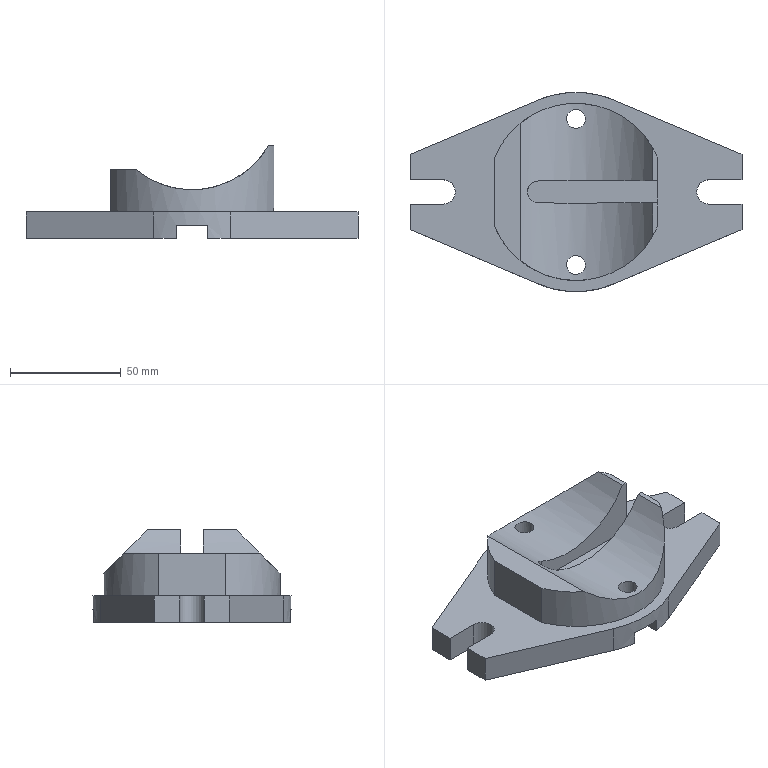Part | NX | features DATUM_CSYS 6, EXTRUDE 5, SKETCH 5, CPROJ 1, DATUM_PLANE 1 | 1 solid | 36 faces | box 150 x 90 x 42 mm | volume 169157 mm3 | plane 26 | cylinder 10 | commonest cylinder face diameters 80 x3 8.5 x2 11 x2 90 x2 10 x1
STEP:
#1=CARTESIAN_POINT('',(34.641,5.,42.));
#2=VERTEX_POINT('',#1);
#3=CARTESIAN_POINT('',(34.641,20.,42.));
#4=VERTEX_POINT('',#3);
#5=CARTESIAN_POINT('',(34.641,-61.,42.));
#6=DIRECTION('',(0.,1.,0.));
#7=VECTOR('',#6,1000.);
#8=LINE('',#5,#7);
#9=EDGE_CURVE('',#2,#4,#8,.T.);
#10=ORIENTED_EDGE('',*,*,#9,.F.);
#11=CARTESIAN_POINT('',(37.,5.,42.));
#12=VERTEX_POINT('',#11);
#13=CARTESIAN_POINT('',(0.,5.,42.));
#14=DIRECTION('',(1.,0.,0.));
#15=VECTOR('',#14,1000.);
#16=LINE('',#13,#15);
#17=EDGE_CURVE('',#2,#12,#16,.T.);
#18=ORIENTED_EDGE('',*,*,#17,.T.);
#19=CARTESIAN_POINT('',(37.,15.199,42.));
#20=VERTEX_POINT('',#19);
#21=CARTESIAN_POINT('',(37.,15.199,42.));
#22=DIRECTION('',(0.,-1.,0.));
#23=VECTOR('',#22,1000.);
#24=LINE('',#21,#23);
#25=EDGE_CURVE('',#20,#12,#24,.T.);
#26=ORIENTED_EDGE('',*,*,#25,.F.);
#27=CARTESIAN_POINT('',(0.,0.,42.));
#28=DIRECTION('',(0.,0.,-1.));
#29=DIRECTION('',(1.,0.,0.));
#30=AXIS2_PLACEMENT_3D('',#27,#28,#29);
#31=CIRCLE('',#30,40.);
#32=EDGE_CURVE('',#4,#20,#31,.T.);
#33=ORIENTED_EDGE('',*,*,#32,.F.);
#34=EDGE_LOOP('',(#10,#18,#26,#33));
#35=FACE_BOUND('',#34,.T.);
#36=CARTESIAN_POINT('',(0.,0.,42.));
#37=DIRECTION('',(0.,0.,-1.));
#38=DIRECTION('',(-1.,0.,0.));
#39=AXIS2_PLACEMENT_3D('',#36,#37,#38);
#40=PLANE('',#39);
#41=ADVANCED_FACE('',(#35),#40,.F.);
#42=CARTESIAN_POINT('',(-7.,-44.452,6.));
#43=VERTEX_POINT('',#42);
#44=CARTESIAN_POINT('',(-7.,-44.452,0.));
#45=VERTEX_POINT('',#44);
#46=CARTESIAN_POINT('',(-7.,-44.452,12.));
#47=DIRECTION('',(0.,0.,-1.));
#48=VECTOR('',#47,1000.);
#49=LINE('',#46,#48);
#50=EDGE_CURVE('',#43,#45,#49,.T.);
#51=ORIENTED_EDGE('',*,*,#50,.F.);
#52=CARTESIAN_POINT('',(7.,-44.452,6.));
#53=VERTEX_POINT('',#52);
#54=CARTESIAN_POINT('',(0.,0.,6.));
#55=DIRECTION('',(0.,0.,-1.));
#56=DIRECTION('',(-1.,0.,0.));
#57=AXIS2_PLACEMENT_3D('',#54,#55,#56);
#58=CIRCLE('',#57,45.);
#59=EDGE_CURVE('',#53,#43,#58,.T.);
#60=ORIENTED_EDGE('',*,*,#59,.F.);
#61=CARTESIAN_POINT('',(7.,-44.452,0.));
#62=VERTEX_POINT('',#61);
#63=CARTESIAN_POINT('',(7.,-44.452,12.));
#64=DIRECTION('',(0.,0.,-1.));
#65=VECTOR('',#64,1000.);
#66=LINE('',#63,#65);
#67=EDGE_CURVE('',#62,#53,#66,.F.);
#68=ORIENTED_EDGE('',*,*,#67,.F.);
#69=CARTESIAN_POINT('',(17.614,-41.41,0.));
#70=VERTEX_POINT('',#69);
#71=CARTESIAN_POINT('',(0.,0.,0.));
#72=DIRECTION('',(0.,0.,1.));
#73=DIRECTION('',(1.,0.,0.));
#74=AXIS2_PLACEMENT_3D('',#71,#72,#73);
#75=CIRCLE('',#74,45.);
#76=EDGE_CURVE('',#62,#70,#75,.T.);
#77=ORIENTED_EDGE('',*,*,#76,.T.);
#78=CARTESIAN_POINT('',(17.614,-41.41,12.));
#79=VERTEX_POINT('',#78);
#80=CARTESIAN_POINT('',(17.614,-41.41,12.));
#81=DIRECTION('',(0.,0.,-1.));
#82=VECTOR('',#81,1000.);
#83=LINE('',#80,#82);
#84=EDGE_CURVE('',#79,#70,#83,.T.);
#85=ORIENTED_EDGE('',*,*,#84,.F.);
#86=CARTESIAN_POINT('',(-17.614,-41.41,12.));
#87=VERTEX_POINT('',#86);
#88=CARTESIAN_POINT('',(0.,0.,12.));
#89=DIRECTION('',(0.,0.,1.));
#90=DIRECTION('',(1.,0.,0.));
#91=AXIS2_PLACEMENT_3D('',#88,#89,#90);
#92=CIRCLE('',#91,45.);
#93=EDGE_CURVE('',#87,#79,#92,.T.);
#94=ORIENTED_EDGE('',*,*,#93,.F.);
#95=CARTESIAN_POINT('',(-17.614,-41.41,0.));
#96=VERTEX_POINT('',#95);
#97=CARTESIAN_POINT('',(-17.614,-41.41,12.));
#98=DIRECTION('',(0.,0.,-1.));
#99=VECTOR('',#98,1000.);
#100=LINE('',#97,#99);
#101=EDGE_CURVE('',#87,#96,#100,.T.);
#102=ORIENTED_EDGE('',*,*,#101,.T.);
#103=CARTESIAN_POINT('',(0.,0.,0.));
#104=DIRECTION('',(0.,0.,1.));
#105=DIRECTION('',(1.,0.,0.));
#106=AXIS2_PLACEMENT_3D('',#103,#104,#105);
#107=CIRCLE('',#106,45.);
#108=EDGE_CURVE('',#96,#45,#107,.T.);
#109=ORIENTED_EDGE('',*,*,#108,.T.);
#110=EDGE_LOOP('',(#51,#60,#68,#77,#85,#94,#102,#109));
#111=FACE_BOUND('',#110,.T.);
#112=CARTESIAN_POINT('',(0.,0.,12.));
#113=DIRECTION('',(0.,0.,-1.));
#114=DIRECTION('',(-1.,0.,0.));
#115=AXIS2_PLACEMENT_3D('',#112,#113,#114);
#116=CYLINDRICAL_SURFACE('',#115,45.);
#117=ADVANCED_FACE('',(#111),#116,.T.);
#118=CARTESIAN_POINT('',(-7.,44.452,0.));
#119=VERTEX_POINT('',#118);
#120=CARTESIAN_POINT('',(-7.,44.452,6.));
#121=VERTEX_POINT('',#120);
#122=CARTESIAN_POINT('',(-7.,44.452,12.));
#123=DIRECTION('',(0.,0.,-1.));
#124=VECTOR('',#123,1000.);
#125=LINE('',#122,#124);
#126=EDGE_CURVE('',#119,#121,#125,.F.);
#127=ORIENTED_EDGE('',*,*,#126,.F.);
#128=CARTESIAN_POINT('',(-17.614,41.41,0.));
#129=VERTEX_POINT('',#128);
#130=CARTESIAN_POINT('',(0.,0.,0.));
#131=DIRECTION('',(0.,0.,1.));
#132=DIRECTION('',(1.,0.,0.));
#133=AXIS2_PLACEMENT_3D('',#130,#131,#132);
#134=CIRCLE('',#133,45.);
#135=EDGE_CURVE('',#119,#129,#134,.T.);
#136=ORIENTED_EDGE('',*,*,#135,.T.);
#137=CARTESIAN_POINT('',(-17.614,41.41,12.));
#138=VERTEX_POINT('',#137);
#139=CARTESIAN_POINT('',(-17.614,41.41,12.));
#140=DIRECTION('',(0.,0.,-1.));
#141=VECTOR('',#140,1000.);
#142=LINE('',#139,#141);
#143=EDGE_CURVE('',#138,#129,#142,.T.);
#144=ORIENTED_EDGE('',*,*,#143,.F.);
#145=CARTESIAN_POINT('',(17.614,41.41,12.));
#146=VERTEX_POINT('',#145);
#147=CARTESIAN_POINT('',(0.,0.,12.));
#148=DIRECTION('',(0.,0.,1.));
#149=DIRECTION('',(1.,0.,0.));
#150=AXIS2_PLACEMENT_3D('',#147,#148,#149);
#151=CIRCLE('',#150,45.);
#152=EDGE_CURVE('',#146,#138,#151,.T.);
#153=ORIENTED_EDGE('',*,*,#152,.F.);
#154=CARTESIAN_POINT('',(17.614,41.41,0.));
#155=VERTEX_POINT('',#154);
#156=CARTESIAN_POINT('',(17.614,41.41,12.));
#157=DIRECTION('',(0.,0.,-1.));
#158=VECTOR('',#157,1000.);
#159=LINE('',#156,#158);
#160=EDGE_CURVE('',#146,#155,#159,.T.);
#161=ORIENTED_EDGE('',*,*,#160,.T.);
#162=CARTESIAN_POINT('',(7.,44.452,0.));
#163=VERTEX_POINT('',#162);
#164=CARTESIAN_POINT('',(0.,0.,0.));
#165=DIRECTION('',(0.,0.,1.));
#166=DIRECTION('',(1.,0.,0.));
#167=AXIS2_PLACEMENT_3D('',#164,#165,#166);
#168=CIRCLE('',#167,45.);
#169=EDGE_CURVE('',#155,#163,#168,.T.);
#170=ORIENTED_EDGE('',*,*,#169,.T.);
#171=CARTESIAN_POINT('',(7.,44.452,6.));
#172=VERTEX_POINT('',#171);
#173=CARTESIAN_POINT('',(7.,44.452,12.));
#174=DIRECTION('',(0.,0.,-1.));
#175=VECTOR('',#174,1000.);
#176=LINE('',#173,#175);
#177=EDGE_CURVE('',#172,#163,#176,.T.);
#178=ORIENTED_EDGE('',*,*,#177,.F.);
#179=CARTESIAN_POINT('',(0.,0.,6.));
#180=DIRECTION('',(0.,0.,-1.));
#181=DIRECTION('',(-1.,0.,0.));
#182=AXIS2_PLACEMENT_3D('',#179,#180,#181);
#183=CIRCLE('',#182,45.);
#184=EDGE_CURVE('',#121,#172,#183,.T.);
#185=ORIENTED_EDGE('',*,*,#184,.F.);
#186=EDGE_LOOP('',(#127,#136,#144,#153,#161,#170,#178,#185));
#187=FACE_BOUND('',#186,.T.);
#188=CARTESIAN_POINT('',(0.,0.,12.));
#189=DIRECTION('',(0.,0.,-1.));
#190=DIRECTION('',(-1.,0.,0.));
#191=AXIS2_PLACEMENT_3D('',#188,#189,#190);
#192=CYLINDRICAL_SURFACE('',#191,45.);
#193=ADVANCED_FACE('',(#187),#192,.T.);
#194=CARTESIAN_POINT('',(-7.,0.,0.));
#195=DIRECTION('',(0.,1.,0.));
#196=VECTOR('',#195,1000.);
#197=LINE('',#194,#196);
#198=EDGE_CURVE('',#45,#119,#197,.T.);
#199=ORIENTED_EDGE('',*,*,#198,.F.);
#200=ORIENTED_EDGE('',*,*,#108,.F.);
#201=CARTESIAN_POINT('',(-75.,-17.,0.));
#202=VERTEX_POINT('',#201);
#203=CARTESIAN_POINT('',(-75.,-17.,0.));
#204=DIRECTION('',(0.9202,-0.3914,0.));
#205=VECTOR('',#204,1000.);
#206=LINE('',#203,#205);
#207=EDGE_CURVE('',#202,#96,#206,.T.);
#208=ORIENTED_EDGE('',*,*,#207,.F.);
#209=CARTESIAN_POINT('',(-75.,-5.5,0.));
#210=VERTEX_POINT('',#209);
#211=CARTESIAN_POINT('',(-75.,-5.5,0.));
#212=DIRECTION('',(0.,-1.,0.));
#213=VECTOR('',#212,1000.);
#214=LINE('',#211,#213);
#215=EDGE_CURVE('',#210,#202,#214,.T.);
#216=ORIENTED_EDGE('',*,*,#215,.F.);
#217=CARTESIAN_POINT('',(-60.,-5.5,0.));
#218=VERTEX_POINT('',#217);
#219=CARTESIAN_POINT('',(-60.,-5.5,0.));
#220=DIRECTION('',(-1.,0.,0.));
#221=VECTOR('',#220,1000.);
#222=LINE('',#219,#221);
#223=EDGE_CURVE('',#218,#210,#222,.T.);
#224=ORIENTED_EDGE('',*,*,#223,.F.);
#225=CARTESIAN_POINT('',(-60.,5.5,0.));
#226=VERTEX_POINT('',#225);
#227=CARTESIAN_POINT('',(-60.,0.,0.));
#228=DIRECTION('',(0.,0.,-1.));
#229=DIRECTION('',(1.,0.,0.));
#230=AXIS2_PLACEMENT_3D('',#227,#228,#229);
#231=CIRCLE('',#230,5.5);
#232=EDGE_CURVE('',#226,#218,#231,.T.);
#233=ORIENTED_EDGE('',*,*,#232,.F.);
#234=CARTESIAN_POINT('',(-75.,5.5,0.));
#235=VERTEX_POINT('',#234);
#236=CARTESIAN_POINT('',(-75.,5.5,0.));
#237=DIRECTION('',(1.,0.,0.));
#238=VECTOR('',#237,1000.);
#239=LINE('',#236,#238);
#240=EDGE_CURVE('',#235,#226,#239,.T.);
#241=ORIENTED_EDGE('',*,*,#240,.F.);
#242=CARTESIAN_POINT('',(-75.,17.,0.));
#243=VERTEX_POINT('',#242);
#244=CARTESIAN_POINT('',(-75.,17.,0.));
#245=DIRECTION('',(0.,-1.,0.));
#246=VECTOR('',#245,1000.);
#247=LINE('',#244,#246);
#248=EDGE_CURVE('',#243,#235,#247,.T.);
#249=ORIENTED_EDGE('',*,*,#248,.F.);
#250=CARTESIAN_POINT('',(-17.614,41.41,0.));
#251=DIRECTION('',(-0.9202,-0.3914,0.));
#252=VECTOR('',#251,1000.);
#253=LINE('',#250,#252);
#254=EDGE_CURVE('',#129,#243,#253,.T.);
#255=ORIENTED_EDGE('',*,*,#254,.F.);
#256=ORIENTED_EDGE('',*,*,#135,.F.);
#257=EDGE_LOOP('',(#199,#200,#208,#216,#224,#233,#241,#249,#255,#256));
#258=FACE_BOUND('',#257,.T.);
#259=CARTESIAN_POINT('',(0.,0.,0.));
#260=DIRECTION('',(0.,0.,1.));
#261=DIRECTION('',(1.,0.,0.));
#262=AXIS2_PLACEMENT_3D('',#259,#260,#261);
#263=PLANE('',#262);
#264=ADVANCED_FACE('',(#258),#263,.F.);
#265=CARTESIAN_POINT('',(7.,0.,0.));
#266=DIRECTION('',(0.,-1.,0.));
#267=VECTOR('',#266,1000.);
#268=LINE('',#265,#267);
#269=EDGE_CURVE('',#163,#62,#268,.T.);
#270=ORIENTED_EDGE('',*,*,#269,.F.);
#271=ORIENTED_EDGE('',*,*,#169,.F.);
#272=CARTESIAN_POINT('',(75.,17.,0.));
#273=VERTEX_POINT('',#272);
#274=CARTESIAN_POINT('',(75.,17.,0.));
#275=DIRECTION('',(-0.9202,0.3914,0.));
#276=VECTOR('',#275,1000.);
#277=LINE('',#274,#276);
#278=EDGE_CURVE('',#273,#155,#277,.T.);
#279=ORIENTED_EDGE('',*,*,#278,.F.);
#280=CARTESIAN_POINT('',(75.,5.5,0.));
#281=VERTEX_POINT('',#280);
#282=CARTESIAN_POINT('',(75.,5.5,0.));
#283=DIRECTION('',(0.,1.,0.));
#284=VECTOR('',#283,1000.);
#285=LINE('',#282,#284);
#286=EDGE_CURVE('',#281,#273,#285,.T.);
#287=ORIENTED_EDGE('',*,*,#286,.F.);
#288=CARTESIAN_POINT('',(60.,5.5,0.));
#289=VERTEX_POINT('',#288);
#290=CARTESIAN_POINT('',(60.,5.5,0.));
#291=DIRECTION('',(1.,0.,0.));
#292=VECTOR('',#291,1000.);
#293=LINE('',#290,#292);
#294=EDGE_CURVE('',#289,#281,#293,.T.);
#295=ORIENTED_EDGE('',*,*,#294,.F.);
#296=CARTESIAN_POINT('',(60.,-5.5,0.));
#297=VERTEX_POINT('',#296);
#298=CARTESIAN_POINT('',(60.,0.,0.));
#299=DIRECTION('',(0.,0.,-1.));
#300=DIRECTION('',(-1.,0.,0.));
#301=AXIS2_PLACEMENT_3D('',#298,#299,#300);
#302=CIRCLE('',#301,5.5);
#303=EDGE_CURVE('',#297,#289,#302,.T.);
#304=ORIENTED_EDGE('',*,*,#303,.F.);
#305=CARTESIAN_POINT('',(75.,-5.5,0.));
#306=VERTEX_POINT('',#305);
#307=CARTESIAN_POINT('',(75.,-5.5,0.));
#308=DIRECTION('',(-1.,0.,0.));
#309=VECTOR('',#308,1000.);
#310=LINE('',#307,#309);
#311=EDGE_CURVE('',#306,#297,#310,.T.);
#312=ORIENTED_EDGE('',*,*,#311,.F.);
#313=CARTESIAN_POINT('',(75.,-17.,0.));
#314=VERTEX_POINT('',#313);
#315=CARTESIAN_POINT('',(75.,-17.,0.));
#316=DIRECTION('',(0.,1.,0.));
#317=VECTOR('',#316,1000.);
#318=LINE('',#315,#317);
#319=EDGE_CURVE('',#314,#306,#318,.T.);
#320=ORIENTED_EDGE('',*,*,#319,.F.);
#321=CARTESIAN_POINT('',(17.614,-41.41,0.));
#322=DIRECTION('',(0.9202,0.3914,0.));
#323=VECTOR('',#322,1000.);
#324=LINE('',#321,#323);
#325=EDGE_CURVE('',#70,#314,#324,.T.);
#326=ORIENTED_EDGE('',*,*,#325,.F.);
#327=ORIENTED_EDGE('',*,*,#76,.F.);
#328=EDGE_LOOP('',(#270,#271,#279,#287,#295,#304,#312,#320,#326,#327));
#329=FACE_BOUND('',#328,.T.);
#330=CARTESIAN_POINT('',(0.,0.,0.));
#331=DIRECTION('',(0.,0.,1.));
#332=DIRECTION('',(1.,0.,0.));
#333=AXIS2_PLACEMENT_3D('',#330,#331,#332);
#334=PLANE('',#333);
#335=ADVANCED_FACE('',(#329),#334,.F.);
#336=CARTESIAN_POINT('',(-37.,-15.199,31.));
#337=VERTEX_POINT('',#336);
#338=CARTESIAN_POINT('',(-37.,-15.199,12.));
#339=VERTEX_POINT('',#338);
#340=CARTESIAN_POINT('',(-37.,-15.199,42.));
#341=DIRECTION('',(0.,0.,-1.));
#342=VECTOR('',#341,1000.);
#343=LINE('',#340,#342);
#344=EDGE_CURVE('',#337,#339,#343,.T.);
#345=ORIENTED_EDGE('',*,*,#344,.F.);
#346=CARTESIAN_POINT('',(-37.,15.199,31.));
#347=VERTEX_POINT('',#346);
#348=CARTESIAN_POINT('',(-37.,-15.199,31.));
#349=DIRECTION('',(0.,1.,0.));
#350=VECTOR('',#349,1000.);
#351=LINE('',#348,#350);
#352=EDGE_CURVE('',#337,#347,#351,.T.);
#353=ORIENTED_EDGE('',*,*,#352,.T.);
#354=CARTESIAN_POINT('',(-37.,15.199,12.));
#355=VERTEX_POINT('',#354);
#356=CARTESIAN_POINT('',(-37.,15.199,42.));
#357=DIRECTION('',(0.,0.,-1.));
#358=VECTOR('',#357,1000.);
#359=LINE('',#356,#358);
#360=EDGE_CURVE('',#347,#355,#359,.T.);
#361=ORIENTED_EDGE('',*,*,#360,.T.);
#362=CARTESIAN_POINT('',(-37.,0.,12.));
#363=DIRECTION('',(0.,-1.,0.));
#364=VECTOR('',#363,1000.);
#365=LINE('',#362,#364);
#366=EDGE_CURVE('',#355,#339,#365,.T.);
#367=ORIENTED_EDGE('',*,*,#366,.T.);
#368=EDGE_LOOP('',(#345,#353,#361,#367));
#369=FACE_BOUND('',#368,.T.);
#370=CARTESIAN_POINT('',(-37.,-15.199,42.));
#371=DIRECTION('',(-1.,0.,0.));
#372=DIRECTION('',(0.,0.,1.));
#373=AXIS2_PLACEMENT_3D('',#370,#371,#372);
#374=PLANE('',#373);
#375=ADVANCED_FACE('',(#369),#374,.T.);
#376=ORIENTED_EDGE('',*,*,#360,.F.);
#377=CARTESIAN_POINT('',(-25.278,31.,31.));
#378=VERTEX_POINT('',#377);
#379=CARTESIAN_POINT('',(0.,0.,31.));
#380=DIRECTION('',(0.,0.,1.));
#381=DIRECTION('',(1.,0.,0.));
#382=AXIS2_PLACEMENT_3D('',#379,#380,#381);
#383=CIRCLE('',#382,40.);
#384=EDGE_CURVE('',#347,#378,#383,.F.);
#385=ORIENTED_EDGE('',*,*,#384,.T.);
#386=CARTESIAN_POINT('',(0.,0.,62.));
#387=DIRECTION('',(0.,-0.7071,-0.7071));
#388=DIRECTION('',(0.,0.7071,-0.7071));
#389=AXIS2_PLACEMENT_3D('',#386,#387,#388);
#390=ELLIPSE('',#389,56.569,40.);
#391=EDGE_CURVE('',#378,#4,#390,.T.);
#392=ORIENTED_EDGE('',*,*,#391,.T.);
#393=ORIENTED_EDGE('',*,*,#32,.T.);
#394=CARTESIAN_POINT('',(37.,15.199,12.));
#395=VERTEX_POINT('',#394);
#396=CARTESIAN_POINT('',(37.,15.199,42.));
#397=DIRECTION('',(0.,0.,-1.));
#398=VECTOR('',#397,1000.);
#399=LINE('',#396,#398);
#400=EDGE_CURVE('',#20,#395,#399,.T.);
#401=ORIENTED_EDGE('',*,*,#400,.T.);
#402=CARTESIAN_POINT('',(0.,0.,12.));
#403=DIRECTION('',(0.,0.,1.));
#404=DIRECTION('',(1.,0.,0.));
#405=AXIS2_PLACEMENT_3D('',#402,#403,#404);
#406=CIRCLE('',#405,40.);
#407=EDGE_CURVE('',#395,#355,#406,.T.);
#408=ORIENTED_EDGE('',*,*,#407,.T.);
#409=EDGE_LOOP('',(#376,#385,#392,#393,#401,#408));
#410=FACE_BOUND('',#409,.T.);
#411=CARTESIAN_POINT('',(0.,0.,42.));
#412=DIRECTION('',(0.,0.,-1.));
#413=DIRECTION('',(-1.,0.,0.));
#414=AXIS2_PLACEMENT_3D('',#411,#412,#413);
#415=CYLINDRICAL_SURFACE('',#414,40.);
#416=ADVANCED_FACE('',(#410),#415,.T.);
#417=CARTESIAN_POINT('',(34.641,-20.,42.));
#418=VERTEX_POINT('',#417);
#419=CARTESIAN_POINT('',(-25.278,-31.,31.));
#420=VERTEX_POINT('',#419);
#421=CARTESIAN_POINT('',(0.,0.,62.));
#422=DIRECTION('',(0.,0.7071,-0.7071));
#423=DIRECTION('',(0.,-0.7071,-0.7071));
#424=AXIS2_PLACEMENT_3D('',#421,#422,#423);
#425=ELLIPSE('',#424,56.569,40.);
#426=EDGE_CURVE('',#418,#420,#425,.T.);
#427=ORIENTED_EDGE('',*,*,#426,.T.);
#428=CARTESIAN_POINT('',(0.,0.,31.));
#429=DIRECTION('',(0.,0.,1.));
#430=DIRECTION('',(1.,0.,0.));
#431=AXIS2_PLACEMENT_3D('',#428,#429,#430);
#432=CIRCLE('',#431,40.);
#433=EDGE_CURVE('',#420,#337,#432,.F.);
#434=ORIENTED_EDGE('',*,*,#433,.T.);
#435=ORIENTED_EDGE('',*,*,#344,.T.);
#436=CARTESIAN_POINT('',(37.,-15.199,12.));
#437=VERTEX_POINT('',#436);
#438=CARTESIAN_POINT('',(0.,0.,12.));
#439=DIRECTION('',(0.,0.,1.));
#440=DIRECTION('',(1.,0.,0.));
#441=AXIS2_PLACEMENT_3D('',#438,#439,#440);
#442=CIRCLE('',#441,40.);
#443=EDGE_CURVE('',#339,#437,#442,.T.);
#444=ORIENTED_EDGE('',*,*,#443,.T.);
#445=CARTESIAN_POINT('',(37.,-15.199,42.));
#446=VERTEX_POINT('',#445);
#447=CARTESIAN_POINT('',(37.,-15.199,42.));
#448=DIRECTION('',(0.,0.,-1.));
#449=VECTOR('',#448,1000.);
#450=LINE('',#447,#449);
#451=EDGE_CURVE('',#446,#437,#450,.T.);
#452=ORIENTED_EDGE('',*,*,#451,.F.);
#453=CARTESIAN_POINT('',(0.,0.,42.));
#454=DIRECTION('',(0.,0.,-1.));
#455=DIRECTION('',(1.,0.,0.));
#456=AXIS2_PLACEMENT_3D('',#453,#454,#455);
#457=CIRCLE('',#456,40.);
#458=EDGE_CURVE('',#446,#418,#457,.T.);
#459=ORIENTED_EDGE('',*,*,#458,.T.);
#460=EDGE_LOOP('',(#427,#434,#435,#444,#452,#459));
#461=FACE_BOUND('',#460,.T.);
#462=CARTESIAN_POINT('',(0.,0.,42.));
#463=DIRECTION('',(0.,0.,-1.));
#464=DIRECTION('',(-1.,0.,0.));
#465=AXIS2_PLACEMENT_3D('',#462,#463,#464);
#466=CYLINDRICAL_SURFACE('',#465,40.);
#467=ADVANCED_FACE('',(#461),#466,.T.);
#468=CARTESIAN_POINT('',(37.,-5.,42.));
#469=VERTEX_POINT('',#468);
#470=CARTESIAN_POINT('',(37.,15.199,42.));
#471=DIRECTION('',(0.,-1.,0.));
#472=VECTOR('',#471,1000.);
#473=LINE('',#470,#472);
#474=EDGE_CURVE('',#469,#446,#473,.T.);
#475=ORIENTED_EDGE('',*,*,#474,.F.);
#476=CARTESIAN_POINT('',(34.641,-5.,42.));
#477=VERTEX_POINT('',#476);
#478=CARTESIAN_POINT('',(0.,-5.,42.));
#479=DIRECTION('',(-1.,0.,0.));
#480=VECTOR('',#479,1000.);
#481=LINE('',#478,#480);
#482=EDGE_CURVE('',#469,#477,#481,.T.);
#483=ORIENTED_EDGE('',*,*,#482,.T.);
#484=CARTESIAN_POINT('',(34.641,-61.,42.));
#485=DIRECTION('',(0.,1.,0.));
#486=VECTOR('',#485,1000.);
#487=LINE('',#484,#486);
#488=EDGE_CURVE('',#418,#477,#487,.T.);
#489=ORIENTED_EDGE('',*,*,#488,.F.);
#490=ORIENTED_EDGE('',*,*,#458,.F.);
#491=EDGE_LOOP('',(#475,#483,#489,#490));
#492=FACE_BOUND('',#491,.T.);
#493=CARTESIAN_POINT('',(0.,0.,42.));
#494=DIRECTION('',(0.,0.,-1.));
#495=DIRECTION('',(-1.,0.,0.));
#496=AXIS2_PLACEMENT_3D('',#493,#494,#495);
#497=PLANE('',#496);
#498=ADVANCED_FACE('',(#492),#497,.F.);
#499=ORIENTED_EDGE('',*,*,#215,.T.);
#500=CARTESIAN_POINT('',(-75.,-17.,12.));
#501=VERTEX_POINT('',#500);
#502=CARTESIAN_POINT('',(-75.,-17.,12.));
#503=DIRECTION('',(0.,0.,-1.));
#504=VECTOR('',#503,1000.);
#505=LINE('',#502,#504);
#506=EDGE_CURVE('',#501,#202,#505,.T.);
#507=ORIENTED_EDGE('',*,*,#506,.F.);
#508=CARTESIAN_POINT('',(-75.,-5.5,12.));
#509=VERTEX_POINT('',#508);
#510=CARTESIAN_POINT('',(-75.,-5.5,12.));
#511=DIRECTION('',(0.,-1.,0.));
#512=VECTOR('',#511,1000.);
#513=LINE('',#510,#512);
#514=EDGE_CURVE('',#509,#501,#513,.T.);
#515=ORIENTED_EDGE('',*,*,#514,.F.);
#516=CARTESIAN_POINT('',(-75.,-5.5,12.));
#517=DIRECTION('',(0.,0.,-1.));
#518=VECTOR('',#517,1000.);
#519=LINE('',#516,#518);
#520=EDGE_CURVE('',#509,#210,#519,.T.);
#521=ORIENTED_EDGE('',*,*,#520,.T.);
#522=EDGE_LOOP('',(#499,#507,#515,#521));
#523=FACE_BOUND('',#522,.T.);
#524=CARTESIAN_POINT('',(-75.,-5.5,12.));
#525=DIRECTION('',(1.,0.,0.));
#526=DIRECTION('',(0.,0.,-1.));
#527=AXIS2_PLACEMENT_3D('',#524,#525,#526);
#528=PLANE('',#527);
#529=ADVANCED_FACE('',(#523),#528,.F.);
#530=ORIENTED_EDGE('',*,*,#207,.T.);
#531=ORIENTED_EDGE('',*,*,#101,.F.);
#532=CARTESIAN_POINT('',(-75.,-17.,12.));
#533=DIRECTION('',(0.9202,-0.3914,0.));
#534=VECTOR('',#533,1000.);
#535=LINE('',#532,#534);
#536=EDGE_CURVE('',#501,#87,#535,.T.);
#537=ORIENTED_EDGE('',*,*,#536,.F.);
#538=ORIENTED_EDGE('',*,*,#506,.T.);
#539=EDGE_LOOP('',(#530,#531,#537,#538));
#540=FACE_BOUND('',#539,.T.);
#541=CARTESIAN_POINT('',(-75.,-17.,12.));
#542=DIRECTION('',(0.3914,0.9202,0.));
#543=DIRECTION('',(-0.9202,0.3914,0.));
#544=AXIS2_PLACEMENT_3D('',#541,#542,#543);
#545=PLANE('',#544);
#546=ADVANCED_FACE('',(#540),#545,.F.);
#547=ORIENTED_EDGE('',*,*,#325,.T.);
#548=CARTESIAN_POINT('',(75.,-17.,12.));
#549=VERTEX_POINT('',#548);
#550=CARTESIAN_POINT('',(75.,-17.,12.));
#551=DIRECTION('',(0.,0.,-1.));
#552=VECTOR('',#551,1000.);
#553=LINE('',#550,#552);
#554=EDGE_CURVE('',#549,#314,#553,.T.);
#555=ORIENTED_EDGE('',*,*,#554,.F.);
#556=CARTESIAN_POINT('',(17.614,-41.41,12.));
#557=DIRECTION('',(0.9202,0.3914,0.));
#558=VECTOR('',#557,1000.);
#559=LINE('',#556,#558);
#560=EDGE_CURVE('',#79,#549,#559,.T.);
#561=ORIENTED_EDGE('',*,*,#560,.F.);
#562=ORIENTED_EDGE('',*,*,#84,.T.);
#563=EDGE_LOOP('',(#547,#555,#561,#562));
#564=FACE_BOUND('',#563,.T.);
#565=CARTESIAN_POINT('',(17.614,-41.41,12.));
#566=DIRECTION('',(-0.3914,0.9202,0.));
#567=DIRECTION('',(-0.9202,-0.3914,0.));
#568=AXIS2_PLACEMENT_3D('',#565,#566,#567);
#569=PLANE('',#568);
#570=ADVANCED_FACE('',(#564),#569,.F.);
#571=ORIENTED_EDGE('',*,*,#319,.T.);
#572=CARTESIAN_POINT('',(75.,-5.5,12.));
#573=VERTEX_POINT('',#572);
#574=CARTESIAN_POINT('',(75.,-5.5,12.));
#575=DIRECTION('',(0.,0.,-1.));
#576=VECTOR('',#575,1000.);
#577=LINE('',#574,#576);
#578=EDGE_CURVE('',#573,#306,#577,.T.);
#579=ORIENTED_EDGE('',*,*,#578,.F.);
#580=CARTESIAN_POINT('',(75.,-17.,12.));
#581=DIRECTION('',(0.,1.,0.));
#582=VECTOR('',#581,1000.);
#583=LINE('',#580,#582);
#584=EDGE_CURVE('',#549,#573,#583,.T.);
#585=ORIENTED_EDGE('',*,*,#584,.F.);
#586=ORIENTED_EDGE('',*,*,#554,.T.);
#587=EDGE_LOOP('',(#571,#579,#585,#586));
#588=FACE_BOUND('',#587,.T.);
#589=CARTESIAN_POINT('',(75.,-17.,12.));
#590=DIRECTION('',(-1.,0.,0.));
#591=DIRECTION('',(0.,0.,1.));
#592=AXIS2_PLACEMENT_3D('',#589,#590,#591);
#593=PLANE('',#592);
#594=ADVANCED_FACE('',(#588),#593,.F.);
#595=ORIENTED_EDGE('',*,*,#311,.T.);
#596=CARTESIAN_POINT('',(60.,-5.5,12.));
#597=VERTEX_POINT('',#596);
#598=CARTESIAN_POINT('',(60.,-5.5,12.));
#599=DIRECTION('',(0.,0.,-1.));
#600=VECTOR('',#599,1000.);
#601=LINE('',#598,#600);
#602=EDGE_CURVE('',#597,#297,#601,.T.);
#603=ORIENTED_EDGE('',*,*,#602,.F.);
#604=CARTESIAN_POINT('',(75.,-5.5,12.));
#605=DIRECTION('',(-1.,0.,0.));
#606=VECTOR('',#605,1000.);
#607=LINE('',#604,#606);
#608=EDGE_CURVE('',#573,#597,#607,.T.);
#609=ORIENTED_EDGE('',*,*,#608,.F.);
#610=ORIENTED_EDGE('',*,*,#578,.T.);
#611=EDGE_LOOP('',(#595,#603,#609,#610));
#612=FACE_BOUND('',#611,.T.);
#613=CARTESIAN_POINT('',(75.,-5.5,12.));
#614=DIRECTION('',(0.,-1.,0.));
#615=DIRECTION('',(0.,0.,-1.));
#616=AXIS2_PLACEMENT_3D('',#613,#614,#615);
#617=PLANE('',#616);
#618=ADVANCED_FACE('',(#612),#617,.F.);
#619=ORIENTED_EDGE('',*,*,#303,.T.);
#620=CARTESIAN_POINT('',(60.,5.5,12.));
#621=VERTEX_POINT('',#620);
#622=CARTESIAN_POINT('',(60.,5.5,12.));
#623=DIRECTION('',(0.,0.,-1.));
#624=VECTOR('',#623,1000.);
#625=LINE('',#622,#624);
#626=EDGE_CURVE('',#621,#289,#625,.T.);
#627=ORIENTED_EDGE('',*,*,#626,.F.);
#628=CARTESIAN_POINT('',(60.,0.,12.));
#629=DIRECTION('',(0.,0.,-1.));
#630=DIRECTION('',(-1.,0.,0.));
#631=AXIS2_PLACEMENT_3D('',#628,#629,#630);
#632=CIRCLE('',#631,5.5);
#633=EDGE_CURVE('',#597,#621,#632,.T.);
#634=ORIENTED_EDGE('',*,*,#633,.F.);
#635=ORIENTED_EDGE('',*,*,#602,.T.);
#636=EDGE_LOOP('',(#619,#627,#634,#635));
#637=FACE_BOUND('',#636,.T.);
#638=CARTESIAN_POINT('',(60.,0.,12.));
#639=DIRECTION('',(0.,0.,-1.));
#640=DIRECTION('',(-1.,0.,0.));
#641=AXIS2_PLACEMENT_3D('',#638,#639,#640);
#642=CYLINDRICAL_SURFACE('',#641,5.5);
#643=ADVANCED_FACE('',(#637),#642,.F.);
#644=ORIENTED_EDGE('',*,*,#294,.T.);
#645=CARTESIAN_POINT('',(75.,5.5,12.));
#646=VERTEX_POINT('',#645);
#647=CARTESIAN_POINT('',(75.,5.5,12.));
#648=DIRECTION('',(0.,0.,-1.));
#649=VECTOR('',#648,1000.);
#650=LINE('',#647,#649);
#651=EDGE_CURVE('',#646,#281,#650,.T.);
#652=ORIENTED_EDGE('',*,*,#651,.F.);
#653=CARTESIAN_POINT('',(60.,5.5,12.));
#654=DIRECTION('',(1.,0.,0.));
#655=VECTOR('',#654,1000.);
#656=LINE('',#653,#655);
#657=EDGE_CURVE('',#621,#646,#656,.T.);
#658=ORIENTED_EDGE('',*,*,#657,.F.);
#659=ORIENTED_EDGE('',*,*,#626,.T.);
#660=EDGE_LOOP('',(#644,#652,#658,#659));
#661=FACE_BOUND('',#660,.T.);
#662=CARTESIAN_POINT('',(60.,5.5,12.));
#663=DIRECTION('',(0.,1.,0.));
#664=DIRECTION('',(0.,0.,1.));
#665=AXIS2_PLACEMENT_3D('',#662,#663,#664);
#666=PLANE('',#665);
#667=ADVANCED_FACE('',(#661),#666,.F.);
#668=ORIENTED_EDGE('',*,*,#286,.T.);
#669=CARTESIAN_POINT('',(75.,17.,12.));
#670=VERTEX_POINT('',#669);
#671=CARTESIAN_POINT('',(75.,17.,12.));
#672=DIRECTION('',(0.,0.,-1.));
#673=VECTOR('',#672,1000.);
#674=LINE('',#671,#673);
#675=EDGE_CURVE('',#670,#273,#674,.T.);
#676=ORIENTED_EDGE('',*,*,#675,.F.);
#677=CARTESIAN_POINT('',(75.,5.5,12.));
#678=DIRECTION('',(0.,1.,0.));
#679=VECTOR('',#678,1000.);
#680=LINE('',#677,#679);
#681=EDGE_CURVE('',#646,#670,#680,.T.);
#682=ORIENTED_EDGE('',*,*,#681,.F.);
#683=ORIENTED_EDGE('',*,*,#651,.T.);
#684=EDGE_LOOP('',(#668,#676,#682,#683));
#685=FACE_BOUND('',#684,.T.);
#686=CARTESIAN_POINT('',(75.,5.5,12.));
#687=DIRECTION('',(-1.,0.,0.));
#688=DIRECTION('',(0.,0.,1.));
#689=AXIS2_PLACEMENT_3D('',#686,#687,#688);
#690=PLANE('',#689);
#691=ADVANCED_FACE('',(#685),#690,.F.);
#692=ORIENTED_EDGE('',*,*,#278,.T.);
#693=ORIENTED_EDGE('',*,*,#160,.F.);
#694=CARTESIAN_POINT('',(75.,17.,12.));
#695=DIRECTION('',(-0.9202,0.3914,0.));
#696=VECTOR('',#695,1000.);
#697=LINE('',#694,#696);
#698=EDGE_CURVE('',#670,#146,#697,.T.);
#699=ORIENTED_EDGE('',*,*,#698,.F.);
#700=ORIENTED_EDGE('',*,*,#675,.T.);
#701=EDGE_LOOP('',(#692,#693,#699,#700));
#702=FACE_BOUND('',#701,.T.);
#703=CARTESIAN_POINT('',(75.,17.,12.));
#704=DIRECTION('',(-0.3914,-0.9202,0.));
#705=DIRECTION('',(0.9202,-0.3914,0.));
#706=AXIS2_PLACEMENT_3D('',#703,#704,#705);
#707=PLANE('',#706);
#708=ADVANCED_FACE('',(#702),#707,.F.);
#709=ORIENTED_EDGE('',*,*,#254,.T.);
#710=CARTESIAN_POINT('',(-75.,17.,12.));
#711=VERTEX_POINT('',#710);
#712=CARTESIAN_POINT('',(-75.,17.,12.));
#713=DIRECTION('',(0.,0.,-1.));
#714=VECTOR('',#713,1000.);
#715=LINE('',#712,#714);
#716=EDGE_CURVE('',#711,#243,#715,.T.);
#717=ORIENTED_EDGE('',*,*,#716,.F.);
#718=CARTESIAN_POINT('',(-17.614,41.41,12.));
#719=DIRECTION('',(-0.9202,-0.3914,0.));
#720=VECTOR('',#719,1000.);
#721=LINE('',#718,#720);
#722=EDGE_CURVE('',#138,#711,#721,.T.);
#723=ORIENTED_EDGE('',*,*,#722,.F.);
#724=ORIENTED_EDGE('',*,*,#143,.T.);
#725=EDGE_LOOP('',(#709,#717,#723,#724));
#726=FACE_BOUND('',#725,.T.);
#727=CARTESIAN_POINT('',(-17.614,41.41,12.));
#728=DIRECTION('',(0.3914,-0.9202,0.));
#729=DIRECTION('',(0.9202,0.3914,0.));
#730=AXIS2_PLACEMENT_3D('',#727,#728,#729);
#731=PLANE('',#730);
#732=ADVANCED_FACE('',(#726),#731,.F.);
#733=ORIENTED_EDGE('',*,*,#248,.T.);
#734=CARTESIAN_POINT('',(-75.,5.5,12.));
#735=VERTEX_POINT('',#734);
#736=CARTESIAN_POINT('',(-75.,5.5,12.));
#737=DIRECTION('',(0.,0.,-1.));
#738=VECTOR('',#737,1000.);
#739=LINE('',#736,#738);
#740=EDGE_CURVE('',#735,#235,#739,.T.);
#741=ORIENTED_EDGE('',*,*,#740,.F.);
#742=CARTESIAN_POINT('',(-75.,17.,12.));
#743=DIRECTION('',(0.,-1.,0.));
#744=VECTOR('',#743,1000.);
#745=LINE('',#742,#744);
#746=EDGE_CURVE('',#711,#735,#745,.T.);
#747=ORIENTED_EDGE('',*,*,#746,.F.);
#748=ORIENTED_EDGE('',*,*,#716,.T.);
#749=EDGE_LOOP('',(#733,#741,#747,#748));
#750=FACE_BOUND('',#749,.T.);
#751=CARTESIAN_POINT('',(-75.,17.,12.));
#752=DIRECTION('',(1.,0.,0.));
#753=DIRECTION('',(0.,0.,-1.));
#754=AXIS2_PLACEMENT_3D('',#751,#752,#753);
#755=PLANE('',#754);
#756=ADVANCED_FACE('',(#750),#755,.F.);
#757=ORIENTED_EDGE('',*,*,#240,.T.);
#758=CARTESIAN_POINT('',(-60.,5.5,12.));
#759=VERTEX_POINT('',#758);
#760=CARTESIAN_POINT('',(-60.,5.5,12.));
#761=DIRECTION('',(0.,0.,-1.));
#762=VECTOR('',#761,1000.);
#763=LINE('',#760,#762);
#764=EDGE_CURVE('',#759,#226,#763,.T.);
#765=ORIENTED_EDGE('',*,*,#764,.F.);
#766=CARTESIAN_POINT('',(-75.,5.5,12.));
#767=DIRECTION('',(1.,0.,0.));
#768=VECTOR('',#767,1000.);
#769=LINE('',#766,#768);
#770=EDGE_CURVE('',#735,#759,#769,.T.);
#771=ORIENTED_EDGE('',*,*,#770,.F.);
#772=ORIENTED_EDGE('',*,*,#740,.T.);
#773=EDGE_LOOP('',(#757,#765,#771,#772));
#774=FACE_BOUND('',#773,.T.);
#775=CARTESIAN_POINT('',(-75.,5.5,12.));
#776=DIRECTION('',(0.,1.,0.));
#777=DIRECTION('',(0.,0.,1.));
#778=AXIS2_PLACEMENT_3D('',#775,#776,#777);
#779=PLANE('',#778);
#780=ADVANCED_FACE('',(#774),#779,.F.);
#781=ORIENTED_EDGE('',*,*,#232,.T.);
#782=CARTESIAN_POINT('',(-60.,-5.5,12.));
#783=VERTEX_POINT('',#782);
#784=CARTESIAN_POINT('',(-60.,-5.5,12.));
#785=DIRECTION('',(0.,0.,-1.));
#786=VECTOR('',#785,1000.);
#787=LINE('',#784,#786);
#788=EDGE_CURVE('',#783,#218,#787,.T.);
#789=ORIENTED_EDGE('',*,*,#788,.F.);
#790=CARTESIAN_POINT('',(-60.,0.,12.));
#791=DIRECTION('',(0.,0.,-1.));
#792=DIRECTION('',(1.,0.,0.));
#793=AXIS2_PLACEMENT_3D('',#790,#791,#792);
#794=CIRCLE('',#793,5.5);
#795=EDGE_CURVE('',#759,#783,#794,.T.);
#796=ORIENTED_EDGE('',*,*,#795,.F.);
#797=ORIENTED_EDGE('',*,*,#764,.T.);
#798=EDGE_LOOP('',(#781,#789,#796,#797));
#799=FACE_BOUND('',#798,.T.);
#800=CARTESIAN_POINT('',(-60.,0.,12.));
#801=DIRECTION('',(0.,0.,-1.));
#802=DIRECTION('',(-1.,0.,0.));
#803=AXIS2_PLACEMENT_3D('',#800,#801,#802);
#804=CYLINDRICAL_SURFACE('',#803,5.5);
#805=ADVANCED_FACE('',(#799),#804,.F.);
#806=ORIENTED_EDGE('',*,*,#223,.T.);
#807=ORIENTED_EDGE('',*,*,#520,.F.);
#808=CARTESIAN_POINT('',(-60.,-5.5,12.));
#809=DIRECTION('',(-1.,0.,0.));
#810=VECTOR('',#809,1000.);
#811=LINE('',#808,#810);
#812=EDGE_CURVE('',#783,#509,#811,.T.);
#813=ORIENTED_EDGE('',*,*,#812,.F.);
#814=ORIENTED_EDGE('',*,*,#788,.T.);
#815=EDGE_LOOP('',(#806,#807,#813,#814));
#816=FACE_BOUND('',#815,.T.);
#817=CARTESIAN_POINT('',(-60.,-5.5,12.));
#818=DIRECTION('',(0.,-1.,0.));
#819=DIRECTION('',(0.,0.,-1.));
#820=AXIS2_PLACEMENT_3D('',#817,#818,#819);
#821=PLANE('',#820);
#822=ADVANCED_FACE('',(#816),#821,.F.);
#823=ORIENTED_EDGE('',*,*,#366,.F.);
#824=ORIENTED_EDGE('',*,*,#407,.F.);
#825=CARTESIAN_POINT('',(37.,0.,12.));
#826=DIRECTION('',(0.,1.,0.));
#827=VECTOR('',#826,1000.);
#828=LINE('',#825,#827);
#829=EDGE_CURVE('',#437,#395,#828,.T.);
#830=ORIENTED_EDGE('',*,*,#829,.F.);
#831=ORIENTED_EDGE('',*,*,#443,.F.);
#832=EDGE_LOOP('',(#823,#824,#830,#831));
#833=FACE_BOUND('',#832,.T.);
#834=ORIENTED_EDGE('',*,*,#514,.T.);
#835=ORIENTED_EDGE('',*,*,#536,.T.);
#836=ORIENTED_EDGE('',*,*,#93,.T.);
#837=ORIENTED_EDGE('',*,*,#560,.T.);
#838=ORIENTED_EDGE('',*,*,#584,.T.);
#839=ORIENTED_EDGE('',*,*,#608,.T.);
#840=ORIENTED_EDGE('',*,*,#633,.T.);
#841=ORIENTED_EDGE('',*,*,#657,.T.);
#842=ORIENTED_EDGE('',*,*,#681,.T.);
#843=ORIENTED_EDGE('',*,*,#698,.T.);
#844=ORIENTED_EDGE('',*,*,#152,.T.);
#845=ORIENTED_EDGE('',*,*,#722,.T.);
#846=ORIENTED_EDGE('',*,*,#746,.T.);
#847=ORIENTED_EDGE('',*,*,#770,.T.);
#848=ORIENTED_EDGE('',*,*,#795,.T.);
#849=ORIENTED_EDGE('',*,*,#812,.T.);
#850=EDGE_LOOP('',(#834,#835,#836,#837,#838,#839,#840,#841,#842,#843,#844,#845,#846,#847,#848,#849));
#851=FACE_BOUND('',#850,.T.);
#852=CARTESIAN_POINT('',(0.,0.,12.));
#853=DIRECTION('',(0.,0.,1.));
#854=DIRECTION('',(1.,0.,0.));
#855=AXIS2_PLACEMENT_3D('',#852,#853,#854);
#856=PLANE('',#855);
#857=ADVANCED_FACE('',(#833,#851),#856,.T.);
#858=CARTESIAN_POINT('',(37.,5.,16.));
#859=VERTEX_POINT('',#858);
#860=CARTESIAN_POINT('',(37.,5.,42.));
#861=DIRECTION('',(0.,0.,1.));
#862=VECTOR('',#861,1000.);
#863=LINE('',#860,#862);
#864=EDGE_CURVE('',#859,#12,#863,.T.);
#865=ORIENTED_EDGE('',*,*,#864,.F.);
#866=CARTESIAN_POINT('',(37.,-5.,16.));
#867=VERTEX_POINT('',#866);
#868=CARTESIAN_POINT('',(37.,15.199,16.));
#869=DIRECTION('',(0.,1.,0.));
#870=VECTOR('',#869,1000.);
#871=LINE('',#868,#870);
#872=EDGE_CURVE('',#867,#859,#871,.T.);
#873=ORIENTED_EDGE('',*,*,#872,.F.);
#874=CARTESIAN_POINT('',(37.,-5.,42.));
#875=DIRECTION('',(0.,0.,-1.));
#876=VECTOR('',#875,1000.);
#877=LINE('',#874,#876);
#878=EDGE_CURVE('',#469,#867,#877,.T.);
#879=ORIENTED_EDGE('',*,*,#878,.F.);
#880=ORIENTED_EDGE('',*,*,#474,.T.);
#881=ORIENTED_EDGE('',*,*,#451,.T.);
#882=ORIENTED_EDGE('',*,*,#829,.T.);
#883=ORIENTED_EDGE('',*,*,#400,.F.);
#884=ORIENTED_EDGE('',*,*,#25,.T.);
#885=EDGE_LOOP('',(#865,#873,#879,#880,#881,#882,#883,#884));
#886=FACE_BOUND('',#885,.T.);
#887=CARTESIAN_POINT('',(37.,15.199,42.));
#888=DIRECTION('',(1.,0.,0.));
#889=DIRECTION('',(0.,0.,-1.));
#890=AXIS2_PLACEMENT_3D('',#887,#888,#889);
#891=PLANE('',#890);
#892=ADVANCED_FACE('',(#886),#891,.T.);
#893=ORIENTED_EDGE('',*,*,#50,.T.);
#894=ORIENTED_EDGE('',*,*,#198,.T.);
#895=ORIENTED_EDGE('',*,*,#126,.T.);
#896=CARTESIAN_POINT('',(-7.,-61.,6.));
#897=DIRECTION('',(0.,1.,0.));
#898=VECTOR('',#897,1000.);
#899=LINE('',#896,#898);
#900=EDGE_CURVE('',#121,#43,#899,.F.);
#901=ORIENTED_EDGE('',*,*,#900,.T.);
#902=EDGE_LOOP('',(#893,#894,#895,#901));
#903=FACE_BOUND('',#902,.T.);
#904=CARTESIAN_POINT('',(-7.,-61.,6.));
#905=DIRECTION('',(1.,0.,0.));
#906=DIRECTION('',(0.,0.,-1.));
#907=AXIS2_PLACEMENT_3D('',#904,#905,#906);
#908=PLANE('',#907);
#909=ADVANCED_FACE('',(#903),#908,.T.);
#910=ORIENTED_EDGE('',*,*,#67,.T.);
#911=CARTESIAN_POINT('',(7.,-61.,6.));
#912=DIRECTION('',(0.,1.,0.));
#913=VECTOR('',#912,1000.);
#914=LINE('',#911,#913);
#915=EDGE_CURVE('',#172,#53,#914,.F.);
#916=ORIENTED_EDGE('',*,*,#915,.F.);
#917=ORIENTED_EDGE('',*,*,#177,.T.);
#918=ORIENTED_EDGE('',*,*,#269,.T.);
#919=EDGE_LOOP('',(#910,#916,#917,#918));
#920=FACE_BOUND('',#919,.T.);
#921=CARTESIAN_POINT('',(7.,-61.,-6.));
#922=DIRECTION('',(-1.,0.,0.));
#923=DIRECTION('',(0.,0.,1.));
#924=AXIS2_PLACEMENT_3D('',#921,#922,#923);
#925=PLANE('',#924);
#926=ADVANCED_FACE('',(#920),#925,.T.);
#927=CARTESIAN_POINT('',(-4.25,33.,6.));
#928=VERTEX_POINT('',#927);
#929=CARTESIAN_POINT('',(0.,33.,6.));
#930=DIRECTION('',(0.,0.,-1.));
#931=DIRECTION('',(-1.,0.,0.));
#932=AXIS2_PLACEMENT_3D('',#929,#930,#931);
#933=CIRCLE('',#932,4.25);
#934=EDGE_CURVE('',#928,#928,#933,.F.);
#935=ORIENTED_EDGE('',*,*,#934,.T.);
#936=EDGE_LOOP('',(#935));
#937=FACE_BOUND('',#936,.T.);
#938=CARTESIAN_POINT('',(-4.25,-33.,6.));
#939=VERTEX_POINT('',#938);
#940=CARTESIAN_POINT('',(0.,-33.,6.));
#941=DIRECTION('',(0.,0.,-1.));
#942=DIRECTION('',(-1.,0.,0.));
#943=AXIS2_PLACEMENT_3D('',#940,#941,#942);
#944=CIRCLE('',#943,4.25);
#945=EDGE_CURVE('',#939,#939,#944,.F.);
#946=ORIENTED_EDGE('',*,*,#945,.T.);
#947=EDGE_LOOP('',(#946));
#948=FACE_BOUND('',#947,.T.);
#949=ORIENTED_EDGE('',*,*,#59,.T.);
#950=ORIENTED_EDGE('',*,*,#900,.F.);
#951=ORIENTED_EDGE('',*,*,#184,.T.);
#952=ORIENTED_EDGE('',*,*,#915,.T.);
#953=EDGE_LOOP('',(#949,#950,#951,#952));
#954=FACE_BOUND('',#953,.T.);
#955=CARTESIAN_POINT('',(7.,-61.,6.));
#956=DIRECTION('',(0.,0.,-1.));
#957=DIRECTION('',(-1.,0.,0.));
#958=AXIS2_PLACEMENT_3D('',#955,#956,#957);
#959=PLANE('',#958);
#960=ADVANCED_FACE('',(#937,#948,#954),#959,.T.);
#961=CARTESIAN_POINT('',(-17.,5.,25.792));
#962=VERTEX_POINT('',#961);
#963=CARTESIAN_POINT('',(0.,5.,62.));
#964=DIRECTION('',(0.,1.,0.));
#965=DIRECTION('',(0.,0.,1.));
#966=AXIS2_PLACEMENT_3D('',#963,#964,#965);
#967=CIRCLE('',#966,40.);
#968=EDGE_CURVE('',#2,#962,#967,.T.);
#969=ORIENTED_EDGE('',*,*,#968,.F.);
#970=ORIENTED_EDGE('',*,*,#9,.T.);
#971=ORIENTED_EDGE('',*,*,#391,.F.);
#972=CARTESIAN_POINT('',(-25.278,-61.,31.));
#973=DIRECTION('',(0.,1.,0.));
#974=VECTOR('',#973,1000.);
#975=LINE('',#972,#974);
#976=EDGE_CURVE('',#378,#420,#975,.F.);
#977=ORIENTED_EDGE('',*,*,#976,.T.);
#978=ORIENTED_EDGE('',*,*,#426,.F.);
#979=ORIENTED_EDGE('',*,*,#488,.T.);
#980=CARTESIAN_POINT('',(-17.,-5.,25.792));
#981=VERTEX_POINT('',#980);
#982=CARTESIAN_POINT('',(0.,-5.,62.));
#983=DIRECTION('',(0.,-1.,0.));
#984=DIRECTION('',(1.,0.,0.));
#985=AXIS2_PLACEMENT_3D('',#982,#983,#984);
#986=CIRCLE('',#985,40.);
#987=EDGE_CURVE('',#981,#477,#986,.T.);
#988=ORIENTED_EDGE('',*,*,#987,.F.);
#989=CARTESIAN_POINT('',(-17.,5.,25.792));
#990=CARTESIAN_POINT('',(-18.279,5.,26.393));
#991=CARTESIAN_POINT('',(-20.11,4.275,27.392));
#992=CARTESIAN_POINT('',(-21.685,2.117,28.384));
#993=CARTESIAN_POINT('',(-22.153,0.01644,28.696));
#994=CARTESIAN_POINT('',(-21.701,-2.085,28.394));
#995=CARTESIAN_POINT('',(-20.122,-4.274,27.399));
#996=CARTESIAN_POINT('',(-18.28,-5.,26.393));
#997=CARTESIAN_POINT('',(-17.,-5.,25.792));
#998=B_SPLINE_CURVE_WITH_KNOTS('',3,(#989,#990,#991,#992,#993,#994,#995,#996,#997),.UNSPECIFIED.,.F.,.F.,(4,1,1,1,1,1,4),(0.,0.004178,0.006267,0.008355,0.01044,0.01253,0.01671),.UNSPECIFIED.);
#999=EDGE_CURVE('',#962,#981,#998,.T.);
#1000=ORIENTED_EDGE('',*,*,#999,.F.);
#1001=EDGE_LOOP('',(#969,#970,#971,#977,#978,#979,#988,#1000));
#1002=FACE_BOUND('',#1001,.T.);
#1003=CARTESIAN_POINT('',(4.25,33.,22.226));
#1004=VERTEX_POINT('',#1003);
#1005=CARTESIAN_POINT('',(3.328,36.334,22.113));
#1006=CARTESIAN_POINT('',(4.711,32.999,22.283));
#1007=CARTESIAN_POINT('',(3.329,29.669,22.113));
#1008=CARTESIAN_POINT('',(0.003708,28.291,21.944));
#1009=CARTESIAN_POINT('',(-3.33,29.668,22.113));
#1010=CARTESIAN_POINT('',(-4.709,32.999,22.283));
#1011=CARTESIAN_POINT('',(-3.334,36.326,22.113));
#1012=CARTESIAN_POINT('',(-0.004486,37.71,21.944));
#1013=CARTESIAN_POINT('',(3.328,36.334,22.113));
#1014=CARTESIAN_POINT('',(4.711,32.999,22.283));
#1015=CARTESIAN_POINT('',(3.329,29.669,22.113));
#1016=B_SPLINE_CURVE_WITH_KNOTS('',3,(#1005,#1006,#1007,#1008,#1009,#1010,#1011,#1012,#1013,#1014,#1015),.UNSPECIFIED.,.T.,.F.,(1,1,1,1,1,1,1,1,1,1,1,1,1,1,1),(-0.009971,-0.006648,-0.003324,0.,0.003324,0.006648,0.009971,0.0133,0.01662,0.01994,0.02327,0.02659,0.02991,0.03324,0.03656),.UNSPECIFIED.);
#1017=EDGE_CURVE('',#1004,#1004,#1016,.T.);
#1018=ORIENTED_EDGE('',*,*,#1017,.T.);
#1019=EDGE_LOOP('',(#1018));
#1020=FACE_BOUND('',#1019,.T.);
#1021=CARTESIAN_POINT('',(4.25,-33.,22.226));
#1022=VERTEX_POINT('',#1021);
#1023=CARTESIAN_POINT('',(3.328,-29.666,22.113));
#1024=CARTESIAN_POINT('',(4.711,-33.001,22.283));
#1025=CARTESIAN_POINT('',(3.329,-36.331,22.113));
#1026=CARTESIAN_POINT('',(0.003708,-37.709,21.944));
#1027=CARTESIAN_POINT('',(-3.33,-36.332,22.113));
#1028=CARTESIAN_POINT('',(-4.709,-33.001,22.283));
#1029=CARTESIAN_POINT('',(-3.334,-29.674,22.113));
#1030=CARTESIAN_POINT('',(-0.004486,-28.29,21.944));
#1031=CARTESIAN_POINT('',(3.328,-29.666,22.113));
#1032=CARTESIAN_POINT('',(4.711,-33.001,22.283));
#1033=CARTESIAN_POINT('',(3.329,-36.331,22.113));
#1034=B_SPLINE_CURVE_WITH_KNOTS('',3,(#1023,#1024,#1025,#1026,#1027,#1028,#1029,#1030,#1031,#1032,#1033),.UNSPECIFIED.,.T.,.F.,(1,1,1,1,1,1,1,1,1,1,1,1,1,1,1),(-0.009971,-0.006648,-0.003324,0.,0.003324,0.006648,0.009971,0.0133,0.01662,0.01994,0.02327,0.02659,0.02991,0.03324,0.03656),.UNSPECIFIED.);
#1035=EDGE_CURVE('',#1022,#1022,#1034,.T.);
#1036=ORIENTED_EDGE('',*,*,#1035,.T.);
#1037=EDGE_LOOP('',(#1036));
#1038=FACE_BOUND('',#1037,.T.);
#1039=CARTESIAN_POINT('',(0.,-61.,62.));
#1040=DIRECTION('',(0.,1.,0.));
#1041=DIRECTION('',(0.,0.,1.));
#1042=AXIS2_PLACEMENT_3D('',#1039,#1040,#1041);
#1043=CYLINDRICAL_SURFACE('',#1042,40.);
#1044=ADVANCED_FACE('',(#1002,#1020,#1038),#1043,.F.);
#1045=ORIENTED_EDGE('',*,*,#352,.F.);
#1046=ORIENTED_EDGE('',*,*,#433,.F.);
#1047=ORIENTED_EDGE('',*,*,#976,.F.);
#1048=ORIENTED_EDGE('',*,*,#384,.F.);
#1049=EDGE_LOOP('',(#1045,#1046,#1047,#1048));
#1050=FACE_BOUND('',#1049,.T.);
#1051=CARTESIAN_POINT('',(-50.,-61.,31.));
#1052=DIRECTION('',(0.,0.,1.));
#1053=DIRECTION('',(1.,0.,0.));
#1054=AXIS2_PLACEMENT_3D('',#1051,#1052,#1053);
#1055=PLANE('',#1054);
#1056=ADVANCED_FACE('',(#1050),#1055,.T.);
#1057=ORIENTED_EDGE('',*,*,#945,.F.);
#1058=EDGE_LOOP('',(#1057));
#1059=FACE_BOUND('',#1058,.T.);
#1060=ORIENTED_EDGE('',*,*,#1035,.F.);
#1061=EDGE_LOOP('',(#1060));
#1062=FACE_BOUND('',#1061,.T.);
#1063=CARTESIAN_POINT('',(0.,-33.,-19.));
#1064=DIRECTION('',(0.,0.,1.));
#1065=DIRECTION('',(1.,0.,0.));
#1066=AXIS2_PLACEMENT_3D('',#1063,#1064,#1065);
#1067=CYLINDRICAL_SURFACE('',#1066,4.25);
#1068=ADVANCED_FACE('',(#1059,#1062),#1067,.F.);
#1069=ORIENTED_EDGE('',*,*,#934,.F.);
#1070=EDGE_LOOP('',(#1069));
#1071=FACE_BOUND('',#1070,.T.);
#1072=ORIENTED_EDGE('',*,*,#1017,.F.);
#1073=EDGE_LOOP('',(#1072));
#1074=FACE_BOUND('',#1073,.T.);
#1075=CARTESIAN_POINT('',(0.,33.,-19.));
#1076=DIRECTION('',(0.,0.,1.));
#1077=DIRECTION('',(1.,0.,0.));
#1078=AXIS2_PLACEMENT_3D('',#1075,#1076,#1077);
#1079=CYLINDRICAL_SURFACE('',#1078,4.25);
#1080=ADVANCED_FACE('',(#1071,#1074),#1079,.F.);
#1081=ORIENTED_EDGE('',*,*,#999,.T.);
#1082=CARTESIAN_POINT('',(-17.,-5.,16.));
#1083=VERTEX_POINT('',#1082);
#1084=CARTESIAN_POINT('',(-17.,-5.,161.));
#1085=DIRECTION('',(0.,0.,-1.));
#1086=VECTOR('',#1085,1000.);
#1087=LINE('',#1084,#1086);
#1088=EDGE_CURVE('',#1083,#981,#1087,.F.);
#1089=ORIENTED_EDGE('',*,*,#1088,.F.);
#1090=CARTESIAN_POINT('',(-17.,5.,16.));
#1091=VERTEX_POINT('',#1090);
#1092=CARTESIAN_POINT('',(-17.,0.,16.));
#1093=DIRECTION('',(0.,0.,-1.));
#1094=DIRECTION('',(1.,0.,0.));
#1095=AXIS2_PLACEMENT_3D('',#1092,#1093,#1094);
#1096=CIRCLE('',#1095,5.);
#1097=EDGE_CURVE('',#1091,#1083,#1096,.F.);
#1098=ORIENTED_EDGE('',*,*,#1097,.F.);
#1099=CARTESIAN_POINT('',(-17.,5.,161.));
#1100=DIRECTION('',(0.,0.,-1.));
#1101=VECTOR('',#1100,1000.);
#1102=LINE('',#1099,#1101);
#1103=EDGE_CURVE('',#1091,#962,#1102,.F.);
#1104=ORIENTED_EDGE('',*,*,#1103,.T.);
#1105=EDGE_LOOP('',(#1081,#1089,#1098,#1104));
#1106=FACE_BOUND('',#1105,.T.);
#1107=CARTESIAN_POINT('',(-17.,0.,161.));
#1108=DIRECTION('',(0.,0.,-1.));
#1109=DIRECTION('',(-1.,0.,0.));
#1110=AXIS2_PLACEMENT_3D('',#1107,#1108,#1109);
#1111=CYLINDRICAL_SURFACE('',#1110,5.);
#1112=ADVANCED_FACE('',(#1106),#1111,.F.);
#1113=ORIENTED_EDGE('',*,*,#864,.T.);
#1114=ORIENTED_EDGE('',*,*,#17,.F.);
#1115=ORIENTED_EDGE('',*,*,#968,.T.);
#1116=ORIENTED_EDGE('',*,*,#1103,.F.);
#1117=CARTESIAN_POINT('',(-17.,5.,16.));
#1118=DIRECTION('',(1.,0.,0.));
#1119=VECTOR('',#1118,1000.);
#1120=LINE('',#1117,#1119);
#1121=EDGE_CURVE('',#859,#1091,#1120,.F.);
#1122=ORIENTED_EDGE('',*,*,#1121,.F.);
#1123=EDGE_LOOP('',(#1113,#1114,#1115,#1116,#1122));
#1124=FACE_BOUND('',#1123,.T.);
#1125=CARTESIAN_POINT('',(-17.,5.,161.));
#1126=DIRECTION('',(0.,1.,0.));
#1127=DIRECTION('',(0.,0.,1.));
#1128=AXIS2_PLACEMENT_3D('',#1125,#1126,#1127);
#1129=PLANE('',#1128);
#1130=ADVANCED_FACE('',(#1124),#1129,.F.);
#1131=ORIENTED_EDGE('',*,*,#878,.T.);
#1132=CARTESIAN_POINT('',(50.709,-5.,16.));
#1133=DIRECTION('',(-1.,0.,0.));
#1134=VECTOR('',#1133,1000.);
#1135=LINE('',#1132,#1134);
#1136=EDGE_CURVE('',#1083,#867,#1135,.F.);
#1137=ORIENTED_EDGE('',*,*,#1136,.F.);
#1138=ORIENTED_EDGE('',*,*,#1088,.T.);
#1139=ORIENTED_EDGE('',*,*,#987,.T.);
#1140=ORIENTED_EDGE('',*,*,#482,.F.);
#1141=EDGE_LOOP('',(#1131,#1137,#1138,#1139,#1140));
#1142=FACE_BOUND('',#1141,.T.);
#1143=CARTESIAN_POINT('',(50.709,-5.,161.));
#1144=DIRECTION('',(0.,-1.,0.));
#1145=DIRECTION('',(1.,0.,0.));
#1146=AXIS2_PLACEMENT_3D('',#1143,#1144,#1145);
#1147=PLANE('',#1146);
#1148=ADVANCED_FACE('',(#1142),#1147,.F.);
#1149=ORIENTED_EDGE('',*,*,#872,.T.);
#1150=ORIENTED_EDGE('',*,*,#1121,.T.);
#1151=ORIENTED_EDGE('',*,*,#1097,.T.);
#1152=ORIENTED_EDGE('',*,*,#1136,.T.);
#1153=EDGE_LOOP('',(#1149,#1150,#1151,#1152));
#1154=FACE_BOUND('',#1153,.T.);
#1155=CARTESIAN_POINT('',(-17.,0.,16.));
#1156=DIRECTION('',(0.,0.,-1.));
#1157=DIRECTION('',(-1.,0.,0.));
#1158=AXIS2_PLACEMENT_3D('',#1155,#1156,#1157);
#1159=PLANE('',#1158);
#1160=ADVANCED_FACE('',(#1154),#1159,.F.);
#1161=CLOSED_SHELL('',(#41,#117,#193,#264,#335,#375,#416,#467,#498,#529,#546,#570,#594,#618,#643,#667,#691,#708,#732,#756,#780,#805,#822,#857,#892,#909,#926,#960,#1044,#1056,#1068,#1080,#1112,#1130,#1148,#1160));
#1162=MANIFOLD_SOLID_BREP('',#1161);
#1163=(LENGTH_UNIT()NAMED_UNIT(*)SI_UNIT(.MILLI.,.METRE.));
#1164=UNCERTAINTY_MEASURE_WITH_UNIT(LENGTH_MEASURE(0.0508),#1163,'','');
#1165=(NAMED_UNIT(*)PLANE_ANGLE_UNIT()SI_UNIT($,.RADIAN.));
#1166=(NAMED_UNIT(*)SI_UNIT($,.STERADIAN.)SOLID_ANGLE_UNIT());
#1167=(GEOMETRIC_REPRESENTATION_CONTEXT(3)GLOBAL_UNCERTAINTY_ASSIGNED_CONTEXT((#1164))GLOBAL_UNIT_ASSIGNED_CONTEXT((#1163,#1165,#1166))REPRESENTATION_CONTEXT('',''));
#1168=ADVANCED_BREP_SHAPE_REPRESENTATION('',(#1162),#1167);